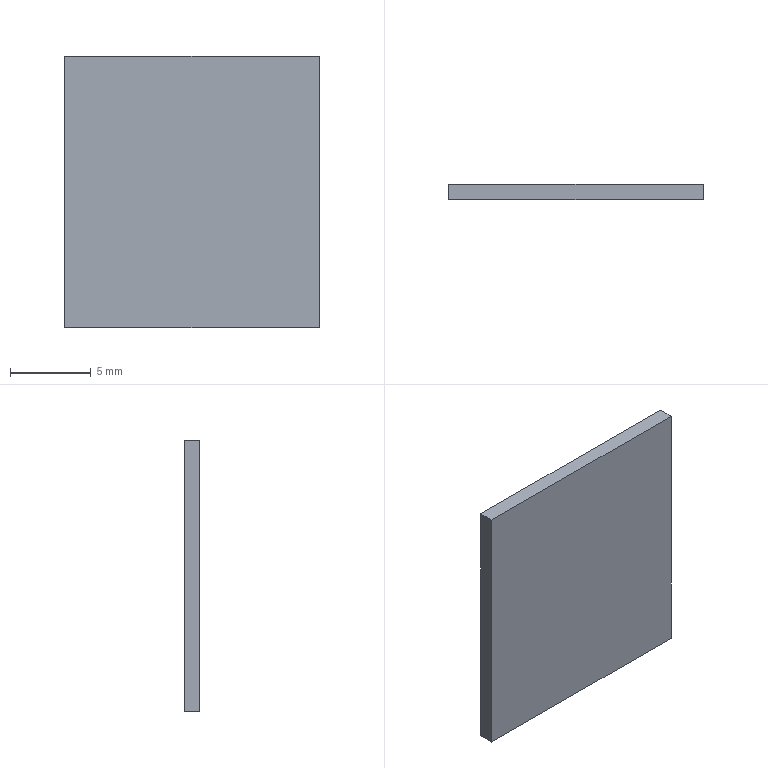Part | SolidWorks | features Extrusion 1, Scale 1 | 1 solid | 6 faces | box 15.76 x 0.95 x 16.86 mm | volume 252.428 mm3 | plane 6
STEP:
#1=CARTESIAN_POINT('',(7.88,0.475,8.43));
#2=VERTEX_POINT('',#1);
#3=CARTESIAN_POINT('',(7.88,0.475,-8.43));
#4=VERTEX_POINT('',#3);
#5=CARTESIAN_POINT('',(7.88,0.475,8.43));
#6=DIRECTION('',(0.,0.,-1.));
#7=VECTOR('',#6,1000.);
#8=LINE('',#5,#7);
#9=EDGE_CURVE('',#2,#4,#8,.T.);
#10=ORIENTED_EDGE('',*,*,#9,.T.);
#11=CARTESIAN_POINT('',(7.88,1.425,-8.43));
#12=VERTEX_POINT('',#11);
#13=CARTESIAN_POINT('',(7.88,1.425,-8.43));
#14=DIRECTION('',(0.,-1.,0.));
#15=VECTOR('',#14,1000.);
#16=LINE('',#13,#15);
#17=EDGE_CURVE('',#12,#4,#16,.T.);
#18=ORIENTED_EDGE('',*,*,#17,.F.);
#19=CARTESIAN_POINT('',(7.88,1.425,8.43));
#20=VERTEX_POINT('',#19);
#21=CARTESIAN_POINT('',(7.88,1.425,8.43));
#22=DIRECTION('',(0.,0.,-1.));
#23=VECTOR('',#22,1000.);
#24=LINE('',#21,#23);
#25=EDGE_CURVE('',#20,#12,#24,.T.);
#26=ORIENTED_EDGE('',*,*,#25,.F.);
#27=CARTESIAN_POINT('',(7.88,1.425,8.43));
#28=DIRECTION('',(0.,-1.,0.));
#29=VECTOR('',#28,1000.);
#30=LINE('',#27,#29);
#31=EDGE_CURVE('',#20,#2,#30,.T.);
#32=ORIENTED_EDGE('',*,*,#31,.T.);
#33=EDGE_LOOP('',(#10,#18,#26,#32));
#34=FACE_OUTER_BOUND('',#33,.T.);
#35=CARTESIAN_POINT('',(7.88,1.425,8.43));
#36=DIRECTION('',(-1.,0.,0.));
#37=DIRECTION('',(0.,0.,1.));
#38=AXIS2_PLACEMENT_3D('',#35,#36,#37);
#39=PLANE('',#38);
#40=ADVANCED_FACE('',(#34),#39,.F.);
#41=CARTESIAN_POINT('',(-7.88,0.475,-8.43));
#42=VERTEX_POINT('',#41);
#43=CARTESIAN_POINT('',(-7.88,0.475,-8.43));
#44=DIRECTION('',(-1.,0.,0.));
#45=VECTOR('',#44,1000.);
#46=LINE('',#43,#45);
#47=EDGE_CURVE('',#4,#42,#46,.T.);
#48=ORIENTED_EDGE('',*,*,#47,.T.);
#49=CARTESIAN_POINT('',(-7.88,1.425,-8.43));
#50=VERTEX_POINT('',#49);
#51=CARTESIAN_POINT('',(-7.88,1.425,-8.43));
#52=DIRECTION('',(0.,-1.,0.));
#53=VECTOR('',#52,1000.);
#54=LINE('',#51,#53);
#55=EDGE_CURVE('',#50,#42,#54,.T.);
#56=ORIENTED_EDGE('',*,*,#55,.F.);
#57=CARTESIAN_POINT('',(-7.88,1.425,-8.43));
#58=DIRECTION('',(-1.,0.,0.));
#59=VECTOR('',#58,1000.);
#60=LINE('',#57,#59);
#61=EDGE_CURVE('',#12,#50,#60,.T.);
#62=ORIENTED_EDGE('',*,*,#61,.F.);
#63=ORIENTED_EDGE('',*,*,#17,.T.);
#64=EDGE_LOOP('',(#48,#56,#62,#63));
#65=FACE_OUTER_BOUND('',#64,.T.);
#66=CARTESIAN_POINT('',(-7.88,1.425,-8.43));
#67=DIRECTION('',(0.,0.,1.));
#68=DIRECTION('',(1.,0.,0.));
#69=AXIS2_PLACEMENT_3D('',#66,#67,#68);
#70=PLANE('',#69);
#71=ADVANCED_FACE('',(#65),#70,.F.);
#72=CARTESIAN_POINT('',(-7.88,0.475,8.43));
#73=VERTEX_POINT('',#72);
#74=CARTESIAN_POINT('',(-7.88,0.475,8.43));
#75=DIRECTION('',(0.,0.,1.));
#76=VECTOR('',#75,1000.);
#77=LINE('',#74,#76);
#78=EDGE_CURVE('',#42,#73,#77,.T.);
#79=ORIENTED_EDGE('',*,*,#78,.T.);
#80=CARTESIAN_POINT('',(-7.88,1.425,8.43));
#81=VERTEX_POINT('',#80);
#82=CARTESIAN_POINT('',(-7.88,1.425,8.43));
#83=DIRECTION('',(0.,-1.,0.));
#84=VECTOR('',#83,1000.);
#85=LINE('',#82,#84);
#86=EDGE_CURVE('',#81,#73,#85,.T.);
#87=ORIENTED_EDGE('',*,*,#86,.F.);
#88=CARTESIAN_POINT('',(-7.88,1.425,8.43));
#89=DIRECTION('',(0.,0.,1.));
#90=VECTOR('',#89,1000.);
#91=LINE('',#88,#90);
#92=EDGE_CURVE('',#50,#81,#91,.T.);
#93=ORIENTED_EDGE('',*,*,#92,.F.);
#94=ORIENTED_EDGE('',*,*,#55,.T.);
#95=EDGE_LOOP('',(#79,#87,#93,#94));
#96=FACE_OUTER_BOUND('',#95,.T.);
#97=CARTESIAN_POINT('',(-7.88,1.425,8.43));
#98=DIRECTION('',(1.,0.,0.));
#99=DIRECTION('',(0.,0.,-1.));
#100=AXIS2_PLACEMENT_3D('',#97,#98,#99);
#101=PLANE('',#100);
#102=ADVANCED_FACE('',(#96),#101,.F.);
#103=CARTESIAN_POINT('',(-7.88,0.475,8.43));
#104=DIRECTION('',(1.,0.,0.));
#105=VECTOR('',#104,1000.);
#106=LINE('',#103,#105);
#107=EDGE_CURVE('',#73,#2,#106,.T.);
#108=ORIENTED_EDGE('',*,*,#107,.T.);
#109=ORIENTED_EDGE('',*,*,#31,.F.);
#110=CARTESIAN_POINT('',(-7.88,1.425,8.43));
#111=DIRECTION('',(1.,0.,0.));
#112=VECTOR('',#111,1000.);
#113=LINE('',#110,#112);
#114=EDGE_CURVE('',#81,#20,#113,.T.);
#115=ORIENTED_EDGE('',*,*,#114,.F.);
#116=ORIENTED_EDGE('',*,*,#86,.T.);
#117=EDGE_LOOP('',(#108,#109,#115,#116));
#118=FACE_OUTER_BOUND('',#117,.T.);
#119=CARTESIAN_POINT('',(-7.88,1.425,8.43));
#120=DIRECTION('',(0.,0.,-1.));
#121=DIRECTION('',(-1.,0.,0.));
#122=AXIS2_PLACEMENT_3D('',#119,#120,#121);
#123=PLANE('',#122);
#124=ADVANCED_FACE('',(#118),#123,.F.);
#125=ORIENTED_EDGE('',*,*,#25,.T.);
#126=ORIENTED_EDGE('',*,*,#61,.T.);
#127=ORIENTED_EDGE('',*,*,#92,.T.);
#128=ORIENTED_EDGE('',*,*,#114,.T.);
#129=EDGE_LOOP('',(#125,#126,#127,#128));
#130=FACE_OUTER_BOUND('',#129,.T.);
#131=CARTESIAN_POINT('',(0.,1.425,0.));
#132=DIRECTION('',(0.,-1.,0.));
#133=DIRECTION('',(0.,0.,-1.));
#134=AXIS2_PLACEMENT_3D('',#131,#132,#133);
#135=PLANE('',#134);
#136=ADVANCED_FACE('',(#130),#135,.F.);
#137=ORIENTED_EDGE('',*,*,#9,.F.);
#138=ORIENTED_EDGE('',*,*,#107,.F.);
#139=ORIENTED_EDGE('',*,*,#78,.F.);
#140=ORIENTED_EDGE('',*,*,#47,.F.);
#141=EDGE_LOOP('',(#137,#138,#139,#140));
#142=FACE_OUTER_BOUND('',#141,.T.);
#143=CARTESIAN_POINT('',(0.,0.475,0.));
#144=DIRECTION('',(0.,-1.,0.));
#145=DIRECTION('',(0.,0.,-1.));
#146=AXIS2_PLACEMENT_3D('',#143,#144,#145);
#147=PLANE('',#146);
#148=ADVANCED_FACE('',(#142),#147,.T.);
#149=CLOSED_SHELL('',(#40,#71,#102,#124,#136,#148));
#150=MANIFOLD_SOLID_BREP('',#149);
#151=CARTESIAN_POINT('',(0.,0.,0.));
#152=DIRECTION('',(0.,0.,1.));
#153=DIRECTION('',(1.,0.,0.));
#154=AXIS2_PLACEMENT_3D('',#151,#152,#153);
#155=(LENGTH_UNIT()NAMED_UNIT(*)SI_UNIT(.MILLI.,.METRE.));
#156=UNCERTAINTY_MEASURE_WITH_UNIT(LENGTH_MEASURE(0.00001),#155,'','');
#157=(NAMED_UNIT(*)PLANE_ANGLE_UNIT()SI_UNIT($,.RADIAN.));
#158=(NAMED_UNIT(*)SI_UNIT($,.STERADIAN.)SOLID_ANGLE_UNIT());
#159=(GEOMETRIC_REPRESENTATION_CONTEXT(3)GLOBAL_UNCERTAINTY_ASSIGNED_CONTEXT((#156))GLOBAL_UNIT_ASSIGNED_CONTEXT((#155,#157,#158))REPRESENTATION_CONTEXT('',''));
#160=ADVANCED_BREP_SHAPE_REPRESENTATION('',(#150,#154),#159);